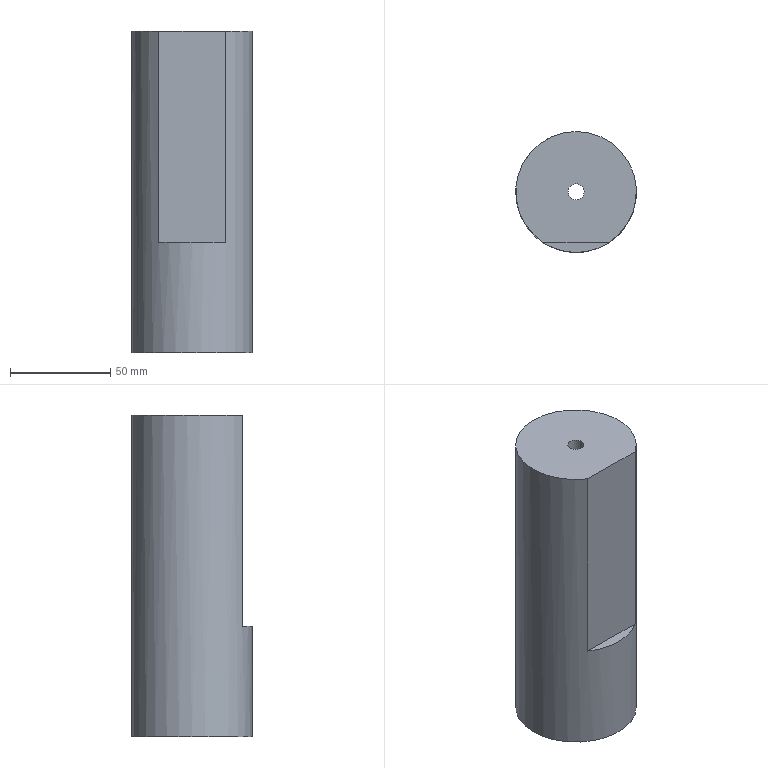Part | NX | features solid 2 | 1 solid | 8 faces | box 60 x 60 x 160 mm | volume 250279 mm3 | plane 5 | cylinder 3 | commonest cylinder face diameters 8 x1 43 x1 60 x1